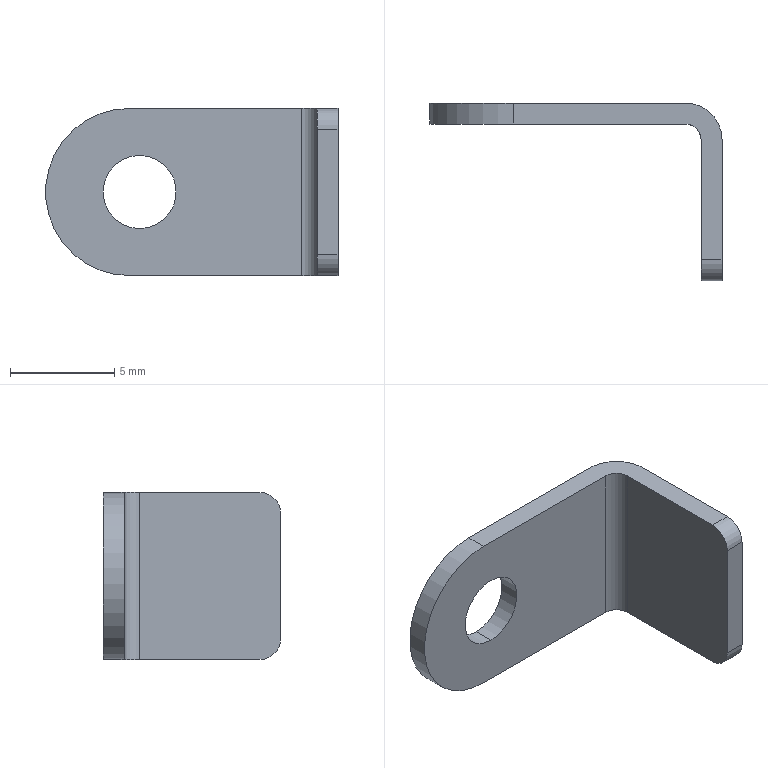Part | SolidWorks | features BaseBody 1 | 1 solid | 14 faces | box 14 x 8.5 x 8 mm | volume 150.836 mm3 | cylinder 7 | plane 7 | commonest cylinder face diameters 2 x2 3.5 x2 1.473 x1 3.473 x1 8 x1
STEP:
#1=CARTESIAN_POINT('',(-2.5,-1.,1.75));
#2=VERTEX_POINT('',#1);
#3=CARTESIAN_POINT('',(-2.5,-1.,-1.75));
#4=VERTEX_POINT('',#3);
#5=CARTESIAN_POINT('',(-2.5,-1.,0.));
#6=DIRECTION('',(0.,-1.,0.));
#7=DIRECTION('',(0.,0.,1.));
#8=AXIS2_PLACEMENT_3D('',#5,#6,#7);
#9=CIRCLE('',#8,1.75);
#10=EDGE_CURVE('',#2,#4,#9,.T.);
#11=ORIENTED_EDGE('',*,*,#10,.T.);
#12=CARTESIAN_POINT('',(-2.5,0.,-1.75));
#13=VERTEX_POINT('',#12);
#14=CARTESIAN_POINT('',(-2.5,-1.,-1.75));
#15=DIRECTION('',(0.,1.,0.));
#16=VECTOR('',#15,1000.);
#17=LINE('',#14,#16);
#18=EDGE_CURVE('',#4,#13,#17,.T.);
#19=ORIENTED_EDGE('',*,*,#18,.T.);
#20=CARTESIAN_POINT('',(-2.5,0.,1.75));
#21=VERTEX_POINT('',#20);
#22=CARTESIAN_POINT('',(-2.5,0.,0.));
#23=DIRECTION('',(0.,-1.,0.));
#24=DIRECTION('',(0.,0.,1.));
#25=AXIS2_PLACEMENT_3D('',#22,#23,#24);
#26=CIRCLE('',#25,1.75);
#27=EDGE_CURVE('',#21,#13,#26,.T.);
#28=ORIENTED_EDGE('',*,*,#27,.F.);
#29=CARTESIAN_POINT('',(-2.5,-1.,1.75));
#30=DIRECTION('',(0.,1.,0.));
#31=VECTOR('',#30,1000.);
#32=LINE('',#29,#31);
#33=EDGE_CURVE('',#2,#21,#32,.T.);
#34=ORIENTED_EDGE('',*,*,#33,.F.);
#35=EDGE_LOOP('',(#11,#19,#28,#34));
#36=FACE_OUTER_BOUND('',#35,.T.);
#37=CARTESIAN_POINT('',(-2.5,-1.,0.));
#38=DIRECTION('',(0.,1.,0.));
#39=DIRECTION('',(0.,0.,1.));
#40=AXIS2_PLACEMENT_3D('',#37,#38,#39);
#41=CYLINDRICAL_SURFACE('',#40,1.75);
#42=ADVANCED_FACE('',(#36),#41,.F.);
#43=CARTESIAN_POINT('',(-3.,-1.,4.));
#44=VERTEX_POINT('',#43);
#45=CARTESIAN_POINT('',(5.263,-1.,4.));
#46=VERTEX_POINT('',#45);
#47=CARTESIAN_POINT('',(-7.,-1.,4.));
#48=DIRECTION('',(1.,0.,0.));
#49=VECTOR('',#48,1000.);
#50=LINE('',#47,#49);
#51=EDGE_CURVE('',#44,#46,#50,.T.);
#52=ORIENTED_EDGE('',*,*,#51,.F.);
#53=CARTESIAN_POINT('',(-3.,-1.,-4.));
#54=VERTEX_POINT('',#53);
#55=CARTESIAN_POINT('',(-3.,-1.,0.));
#56=DIRECTION('',(0.,1.,0.));
#57=DIRECTION('',(0.,0.,1.));
#58=AXIS2_PLACEMENT_3D('',#55,#56,#57);
#59=CIRCLE('',#58,4.);
#60=EDGE_CURVE('',#54,#44,#59,.T.);
#61=ORIENTED_EDGE('',*,*,#60,.F.);
#62=CARTESIAN_POINT('',(5.263,-1.,-4.));
#63=VERTEX_POINT('',#62);
#64=CARTESIAN_POINT('',(-7.,-1.,-4.));
#65=DIRECTION('',(-1.,0.,0.));
#66=VECTOR('',#65,1000.);
#67=LINE('',#64,#66);
#68=EDGE_CURVE('',#63,#54,#67,.T.);
#69=ORIENTED_EDGE('',*,*,#68,.F.);
#70=CARTESIAN_POINT('',(5.263,-1.,4.));
#71=DIRECTION('',(0.,0.,-1.));
#72=VECTOR('',#71,1000.);
#73=LINE('',#70,#72);
#74=EDGE_CURVE('',#46,#63,#73,.T.);
#75=ORIENTED_EDGE('',*,*,#74,.F.);
#76=EDGE_LOOP('',(#52,#61,#69,#75));
#77=FACE_OUTER_BOUND('',#76,.T.);
#78=ORIENTED_EDGE('',*,*,#10,.F.);
#79=CARTESIAN_POINT('',(-2.5,-1.,0.));
#80=DIRECTION('',(0.,-1.,0.));
#81=DIRECTION('',(0.,0.,1.));
#82=AXIS2_PLACEMENT_3D('',#79,#80,#81);
#83=CIRCLE('',#82,1.75);
#84=EDGE_CURVE('',#4,#2,#83,.T.);
#85=ORIENTED_EDGE('',*,*,#84,.F.);
#86=EDGE_LOOP('',(#78,#85));
#87=FACE_BOUND('',#86,.T.);
#88=CARTESIAN_POINT('',(-7.,-1.,4.));
#89=DIRECTION('',(0.,1.,0.));
#90=DIRECTION('',(0.,0.,1.));
#91=AXIS2_PLACEMENT_3D('',#88,#89,#90);
#92=PLANE('',#91);
#93=ADVANCED_FACE('',(#77,#87),#92,.F.);
#94=CARTESIAN_POINT('',(6.,-1.737,-4.));
#95=VERTEX_POINT('',#94);
#96=CARTESIAN_POINT('',(5.263,-1.737,-4.));
#97=DIRECTION('',(0.,0.,1.));
#98=DIRECTION('',(1.,0.,0.));
#99=AXIS2_PLACEMENT_3D('',#96,#97,#98);
#100=CIRCLE('',#99,0.7366);
#101=EDGE_CURVE('',#95,#63,#100,.T.);
#102=ORIENTED_EDGE('',*,*,#101,.F.);
#103=CARTESIAN_POINT('',(6.,-1.737,4.));
#104=VERTEX_POINT('',#103);
#105=CARTESIAN_POINT('',(6.,-1.737,4.));
#106=DIRECTION('',(0.,0.,-1.));
#107=VECTOR('',#106,1000.);
#108=LINE('',#105,#107);
#109=EDGE_CURVE('',#104,#95,#108,.T.);
#110=ORIENTED_EDGE('',*,*,#109,.F.);
#111=CARTESIAN_POINT('',(5.263,-1.737,4.));
#112=DIRECTION('',(0.,0.,1.));
#113=DIRECTION('',(1.,0.,0.));
#114=AXIS2_PLACEMENT_3D('',#111,#112,#113);
#115=CIRCLE('',#114,0.7366);
#116=EDGE_CURVE('',#104,#46,#115,.T.);
#117=ORIENTED_EDGE('',*,*,#116,.T.);
#118=ORIENTED_EDGE('',*,*,#74,.T.);
#119=EDGE_LOOP('',(#102,#110,#117,#118));
#120=FACE_OUTER_BOUND('',#119,.T.);
#121=CARTESIAN_POINT('',(5.263,-1.737,4.));
#122=DIRECTION('',(0.,0.,1.));
#123=DIRECTION('',(1.,0.,0.));
#124=AXIS2_PLACEMENT_3D('',#121,#122,#123);
#125=CYLINDRICAL_SURFACE('',#124,0.7366);
#126=ADVANCED_FACE('',(#120),#125,.F.);
#127=CARTESIAN_POINT('',(-3.,0.,4.));
#128=VERTEX_POINT('',#127);
#129=CARTESIAN_POINT('',(5.263,0.,4.));
#130=VERTEX_POINT('',#129);
#131=CARTESIAN_POINT('',(0.,0.,4.));
#132=DIRECTION('',(1.,0.,0.));
#133=VECTOR('',#132,1000.);
#134=LINE('',#131,#133);
#135=EDGE_CURVE('',#128,#130,#134,.T.);
#136=ORIENTED_EDGE('',*,*,#135,.F.);
#137=CARTESIAN_POINT('',(-3.,0.,4.));
#138=DIRECTION('',(0.,1.,0.));
#139=VECTOR('',#138,1000.);
#140=LINE('',#137,#139);
#141=EDGE_CURVE('',#44,#128,#140,.T.);
#142=ORIENTED_EDGE('',*,*,#141,.F.);
#143=ORIENTED_EDGE('',*,*,#51,.T.);
#144=ORIENTED_EDGE('',*,*,#116,.F.);
#145=CARTESIAN_POINT('',(6.,-7.5,4.));
#146=VERTEX_POINT('',#145);
#147=CARTESIAN_POINT('',(6.,0.,4.));
#148=DIRECTION('',(0.,1.,0.));
#149=VECTOR('',#148,1000.);
#150=LINE('',#147,#149);
#151=EDGE_CURVE('',#146,#104,#150,.T.);
#152=ORIENTED_EDGE('',*,*,#151,.F.);
#153=CARTESIAN_POINT('',(7.,-7.5,4.));
#154=VERTEX_POINT('',#153);
#155=CARTESIAN_POINT('',(7.,-7.5,4.));
#156=DIRECTION('',(-1.,0.,0.));
#157=VECTOR('',#156,1000.);
#158=LINE('',#155,#157);
#159=EDGE_CURVE('',#154,#146,#158,.T.);
#160=ORIENTED_EDGE('',*,*,#159,.F.);
#161=CARTESIAN_POINT('',(7.,-1.737,4.));
#162=VERTEX_POINT('',#161);
#163=CARTESIAN_POINT('',(7.,-8.5,4.));
#164=DIRECTION('',(0.,-1.,0.));
#165=VECTOR('',#164,1000.);
#166=LINE('',#163,#165);
#167=EDGE_CURVE('',#162,#154,#166,.T.);
#168=ORIENTED_EDGE('',*,*,#167,.F.);
#169=CARTESIAN_POINT('',(5.263,-1.737,4.));
#170=DIRECTION('',(0.,0.,-1.));
#171=DIRECTION('',(1.,0.,0.));
#172=AXIS2_PLACEMENT_3D('',#169,#170,#171);
#173=CIRCLE('',#172,1.737);
#174=EDGE_CURVE('',#130,#162,#173,.T.);
#175=ORIENTED_EDGE('',*,*,#174,.F.);
#176=EDGE_LOOP('',(#136,#142,#143,#144,#152,#160,#168,#175));
#177=FACE_OUTER_BOUND('',#176,.T.);
#178=CARTESIAN_POINT('',(0.,0.,4.));
#179=DIRECTION('',(0.,0.,-1.));
#180=DIRECTION('',(-1.,0.,0.));
#181=AXIS2_PLACEMENT_3D('',#178,#179,#180);
#182=PLANE('',#181);
#183=ADVANCED_FACE('',(#177),#182,.F.);
#184=ORIENTED_EDGE('',*,*,#141,.T.);
#185=CARTESIAN_POINT('',(-3.,0.,-4.));
#186=VERTEX_POINT('',#185);
#187=CARTESIAN_POINT('',(-3.,0.,0.));
#188=DIRECTION('',(0.,-1.,0.));
#189=DIRECTION('',(0.,0.,-1.));
#190=AXIS2_PLACEMENT_3D('',#187,#188,#189);
#191=CIRCLE('',#190,4.);
#192=EDGE_CURVE('',#128,#186,#191,.T.);
#193=ORIENTED_EDGE('',*,*,#192,.T.);
#194=CARTESIAN_POINT('',(-3.,0.,-4.));
#195=DIRECTION('',(0.,-1.,0.));
#196=VECTOR('',#195,1000.);
#197=LINE('',#194,#196);
#198=EDGE_CURVE('',#186,#54,#197,.T.);
#199=ORIENTED_EDGE('',*,*,#198,.T.);
#200=ORIENTED_EDGE('',*,*,#60,.T.);
#201=EDGE_LOOP('',(#184,#193,#199,#200));
#202=FACE_OUTER_BOUND('',#201,.T.);
#203=CARTESIAN_POINT('',(-3.,-1.,0.));
#204=DIRECTION('',(0.,-1.,0.));
#205=DIRECTION('',(0.,0.,-1.));
#206=AXIS2_PLACEMENT_3D('',#203,#204,#205);
#207=CYLINDRICAL_SURFACE('',#206,4.);
#208=ADVANCED_FACE('',(#202),#207,.T.);
#209=ORIENTED_EDGE('',*,*,#198,.F.);
#210=CARTESIAN_POINT('',(5.263,0.,-4.));
#211=VERTEX_POINT('',#210);
#212=CARTESIAN_POINT('',(0.,0.,-4.));
#213=DIRECTION('',(1.,0.,0.));
#214=VECTOR('',#213,1000.);
#215=LINE('',#212,#214);
#216=EDGE_CURVE('',#186,#211,#215,.T.);
#217=ORIENTED_EDGE('',*,*,#216,.T.);
#218=CARTESIAN_POINT('',(7.,-1.737,-4.));
#219=VERTEX_POINT('',#218);
#220=CARTESIAN_POINT('',(5.263,-1.737,-4.));
#221=DIRECTION('',(0.,0.,1.));
#222=DIRECTION('',(1.,0.,0.));
#223=AXIS2_PLACEMENT_3D('',#220,#221,#222);
#224=CIRCLE('',#223,1.737);
#225=EDGE_CURVE('',#219,#211,#224,.T.);
#226=ORIENTED_EDGE('',*,*,#225,.F.);
#227=CARTESIAN_POINT('',(7.,-7.5,-4.));
#228=VERTEX_POINT('',#227);
#229=CARTESIAN_POINT('',(7.,-1.,-4.));
#230=DIRECTION('',(0.,1.,0.));
#231=VECTOR('',#230,1000.);
#232=LINE('',#229,#231);
#233=EDGE_CURVE('',#228,#219,#232,.T.);
#234=ORIENTED_EDGE('',*,*,#233,.F.);
#235=CARTESIAN_POINT('',(6.,-7.5,-4.));
#236=VERTEX_POINT('',#235);
#237=CARTESIAN_POINT('',(7.,-7.5,-4.));
#238=DIRECTION('',(1.,0.,0.));
#239=VECTOR('',#238,1000.);
#240=LINE('',#237,#239);
#241=EDGE_CURVE('',#236,#228,#240,.T.);
#242=ORIENTED_EDGE('',*,*,#241,.F.);
#243=CARTESIAN_POINT('',(6.,0.,-4.));
#244=DIRECTION('',(0.,-1.,0.));
#245=VECTOR('',#244,1000.);
#246=LINE('',#243,#245);
#247=EDGE_CURVE('',#95,#236,#246,.T.);
#248=ORIENTED_EDGE('',*,*,#247,.F.);
#249=ORIENTED_EDGE('',*,*,#101,.T.);
#250=ORIENTED_EDGE('',*,*,#68,.T.);
#251=EDGE_LOOP('',(#209,#217,#226,#234,#242,#248,#249,#250));
#252=FACE_OUTER_BOUND('',#251,.T.);
#253=CARTESIAN_POINT('',(0.,0.,-4.));
#254=DIRECTION('',(0.,0.,-1.));
#255=DIRECTION('',(-1.,0.,0.));
#256=AXIS2_PLACEMENT_3D('',#253,#254,#255);
#257=PLANE('',#256);
#258=ADVANCED_FACE('',(#252),#257,.T.);
#259=ORIENTED_EDGE('',*,*,#18,.F.);
#260=ORIENTED_EDGE('',*,*,#84,.T.);
#261=ORIENTED_EDGE('',*,*,#33,.T.);
#262=CARTESIAN_POINT('',(-2.5,0.,0.));
#263=DIRECTION('',(0.,-1.,0.));
#264=DIRECTION('',(0.,0.,1.));
#265=AXIS2_PLACEMENT_3D('',#262,#263,#264);
#266=CIRCLE('',#265,1.75);
#267=EDGE_CURVE('',#13,#21,#266,.T.);
#268=ORIENTED_EDGE('',*,*,#267,.F.);
#269=EDGE_LOOP('',(#259,#260,#261,#268));
#270=FACE_OUTER_BOUND('',#269,.T.);
#271=CARTESIAN_POINT('',(-2.5,-1.,0.));
#272=DIRECTION('',(0.,1.,0.));
#273=DIRECTION('',(0.,0.,1.));
#274=AXIS2_PLACEMENT_3D('',#271,#272,#273);
#275=CYLINDRICAL_SURFACE('',#274,1.75);
#276=ADVANCED_FACE('',(#270),#275,.F.);
#277=ORIENTED_EDGE('',*,*,#247,.T.);
#278=CARTESIAN_POINT('',(6.,-8.5,-3.));
#279=VERTEX_POINT('',#278);
#280=CARTESIAN_POINT('',(6.,-7.5,-3.));
#281=DIRECTION('',(-1.,0.,0.));
#282=DIRECTION('',(0.,-1.,0.));
#283=AXIS2_PLACEMENT_3D('',#280,#281,#282);
#284=CIRCLE('',#283,1.);
#285=EDGE_CURVE('',#236,#279,#284,.T.);
#286=ORIENTED_EDGE('',*,*,#285,.T.);
#287=CARTESIAN_POINT('',(6.,-8.5,3.));
#288=VERTEX_POINT('',#287);
#289=CARTESIAN_POINT('',(6.,-8.5,0.));
#290=DIRECTION('',(0.,0.,1.));
#291=VECTOR('',#290,1000.);
#292=LINE('',#289,#291);
#293=EDGE_CURVE('',#279,#288,#292,.T.);
#294=ORIENTED_EDGE('',*,*,#293,.T.);
#295=CARTESIAN_POINT('',(6.,-7.5,3.));
#296=DIRECTION('',(-1.,0.,0.));
#297=DIRECTION('',(0.,-1.,0.));
#298=AXIS2_PLACEMENT_3D('',#295,#296,#297);
#299=CIRCLE('',#298,1.);
#300=EDGE_CURVE('',#288,#146,#299,.T.);
#301=ORIENTED_EDGE('',*,*,#300,.T.);
#302=ORIENTED_EDGE('',*,*,#151,.T.);
#303=ORIENTED_EDGE('',*,*,#109,.T.);
#304=EDGE_LOOP('',(#277,#286,#294,#301,#302,#303));
#305=FACE_OUTER_BOUND('',#304,.T.);
#306=CARTESIAN_POINT('',(6.,0.,0.));
#307=DIRECTION('',(-1.,0.,0.));
#308=DIRECTION('',(0.,-1.,0.));
#309=AXIS2_PLACEMENT_3D('',#306,#307,#308);
#310=PLANE('',#309);
#311=ADVANCED_FACE('',(#305),#310,.T.);
#312=ORIENTED_EDGE('',*,*,#216,.F.);
#313=ORIENTED_EDGE('',*,*,#192,.F.);
#314=ORIENTED_EDGE('',*,*,#135,.T.);
#315=CARTESIAN_POINT('',(5.263,0.,4.));
#316=DIRECTION('',(0.,0.,-1.));
#317=VECTOR('',#316,1000.);
#318=LINE('',#315,#317);
#319=EDGE_CURVE('',#130,#211,#318,.T.);
#320=ORIENTED_EDGE('',*,*,#319,.T.);
#321=EDGE_LOOP('',(#312,#313,#314,#320));
#322=FACE_OUTER_BOUND('',#321,.T.);
#323=ORIENTED_EDGE('',*,*,#27,.T.);
#324=ORIENTED_EDGE('',*,*,#267,.T.);
#325=EDGE_LOOP('',(#323,#324));
#326=FACE_BOUND('',#325,.T.);
#327=CARTESIAN_POINT('',(-7.,0.,4.));
#328=DIRECTION('',(0.,1.,0.));
#329=DIRECTION('',(0.,0.,1.));
#330=AXIS2_PLACEMENT_3D('',#327,#328,#329);
#331=PLANE('',#330);
#332=ADVANCED_FACE('',(#322,#326),#331,.T.);
#333=ORIENTED_EDGE('',*,*,#285,.F.);
#334=ORIENTED_EDGE('',*,*,#241,.T.);
#335=CARTESIAN_POINT('',(7.,-8.5,-3.));
#336=VERTEX_POINT('',#335);
#337=CARTESIAN_POINT('',(7.,-7.5,-3.));
#338=DIRECTION('',(-1.,0.,0.));
#339=DIRECTION('',(0.,-1.,0.));
#340=AXIS2_PLACEMENT_3D('',#337,#338,#339);
#341=CIRCLE('',#340,1.);
#342=EDGE_CURVE('',#228,#336,#341,.T.);
#343=ORIENTED_EDGE('',*,*,#342,.T.);
#344=CARTESIAN_POINT('',(7.,-8.5,-3.));
#345=DIRECTION('',(-1.,0.,0.));
#346=VECTOR('',#345,1000.);
#347=LINE('',#344,#346);
#348=EDGE_CURVE('',#336,#279,#347,.T.);
#349=ORIENTED_EDGE('',*,*,#348,.T.);
#350=EDGE_LOOP('',(#333,#334,#343,#349));
#351=FACE_OUTER_BOUND('',#350,.T.);
#352=CARTESIAN_POINT('',(7.,-7.5,-3.));
#353=DIRECTION('',(-1.,0.,0.));
#354=DIRECTION('',(0.,-1.,0.));
#355=AXIS2_PLACEMENT_3D('',#352,#353,#354);
#356=CYLINDRICAL_SURFACE('',#355,1.);
#357=ADVANCED_FACE('',(#351),#356,.T.);
#358=ORIENTED_EDGE('',*,*,#300,.F.);
#359=CARTESIAN_POINT('',(7.,-8.5,3.));
#360=VERTEX_POINT('',#359);
#361=CARTESIAN_POINT('',(7.,-8.5,3.));
#362=DIRECTION('',(1.,0.,0.));
#363=VECTOR('',#362,1000.);
#364=LINE('',#361,#363);
#365=EDGE_CURVE('',#288,#360,#364,.T.);
#366=ORIENTED_EDGE('',*,*,#365,.T.);
#367=CARTESIAN_POINT('',(7.,-7.5,3.));
#368=DIRECTION('',(-1.,0.,0.));
#369=DIRECTION('',(0.,-1.,0.));
#370=AXIS2_PLACEMENT_3D('',#367,#368,#369);
#371=CIRCLE('',#370,1.);
#372=EDGE_CURVE('',#360,#154,#371,.T.);
#373=ORIENTED_EDGE('',*,*,#372,.T.);
#374=ORIENTED_EDGE('',*,*,#159,.T.);
#375=EDGE_LOOP('',(#358,#366,#373,#374));
#376=FACE_OUTER_BOUND('',#375,.T.);
#377=CARTESIAN_POINT('',(7.,-7.5,3.));
#378=DIRECTION('',(-1.,0.,0.));
#379=DIRECTION('',(0.,-1.,0.));
#380=AXIS2_PLACEMENT_3D('',#377,#378,#379);
#381=CYLINDRICAL_SURFACE('',#380,1.);
#382=ADVANCED_FACE('',(#376),#381,.T.);
#383=ORIENTED_EDGE('',*,*,#365,.F.);
#384=ORIENTED_EDGE('',*,*,#293,.F.);
#385=ORIENTED_EDGE('',*,*,#348,.F.);
#386=CARTESIAN_POINT('',(7.,-8.5,-4.));
#387=DIRECTION('',(0.,0.,-1.));
#388=VECTOR('',#387,1000.);
#389=LINE('',#386,#388);
#390=EDGE_CURVE('',#360,#336,#389,.T.);
#391=ORIENTED_EDGE('',*,*,#390,.F.);
#392=EDGE_LOOP('',(#383,#384,#385,#391));
#393=FACE_OUTER_BOUND('',#392,.T.);
#394=CARTESIAN_POINT('',(7.,-8.5,-4.));
#395=DIRECTION('',(0.,1.,0.));
#396=DIRECTION('',(-1.,0.,0.));
#397=AXIS2_PLACEMENT_3D('',#394,#395,#396);
#398=PLANE('',#397);
#399=ADVANCED_FACE('',(#393),#398,.F.);
#400=CARTESIAN_POINT('',(7.,-1.737,4.));
#401=DIRECTION('',(0.,0.,-1.));
#402=VECTOR('',#401,1000.);
#403=LINE('',#400,#402);
#404=EDGE_CURVE('',#162,#219,#403,.T.);
#405=ORIENTED_EDGE('',*,*,#404,.T.);
#406=ORIENTED_EDGE('',*,*,#225,.T.);
#407=ORIENTED_EDGE('',*,*,#319,.F.);
#408=ORIENTED_EDGE('',*,*,#174,.T.);
#409=EDGE_LOOP('',(#405,#406,#407,#408));
#410=FACE_OUTER_BOUND('',#409,.T.);
#411=CARTESIAN_POINT('',(5.263,-1.737,4.));
#412=DIRECTION('',(0.,0.,1.));
#413=DIRECTION('',(1.,0.,0.));
#414=AXIS2_PLACEMENT_3D('',#411,#412,#413);
#415=CYLINDRICAL_SURFACE('',#414,1.737);
#416=ADVANCED_FACE('',(#410),#415,.T.);
#417=ORIENTED_EDGE('',*,*,#372,.F.);
#418=ORIENTED_EDGE('',*,*,#390,.T.);
#419=ORIENTED_EDGE('',*,*,#342,.F.);
#420=ORIENTED_EDGE('',*,*,#233,.T.);
#421=ORIENTED_EDGE('',*,*,#404,.F.);
#422=ORIENTED_EDGE('',*,*,#167,.T.);
#423=EDGE_LOOP('',(#417,#418,#419,#420,#421,#422));
#424=FACE_OUTER_BOUND('',#423,.T.);
#425=CARTESIAN_POINT('',(7.,0.,0.));
#426=DIRECTION('',(-1.,0.,0.));
#427=DIRECTION('',(0.,-1.,0.));
#428=AXIS2_PLACEMENT_3D('',#425,#426,#427);
#429=PLANE('',#428);
#430=ADVANCED_FACE('',(#424),#429,.F.);
#431=CLOSED_SHELL('',(#42,#93,#126,#183,#208,#258,#276,#311,#332,#357,#382,#399,#416,#430));
#432=MANIFOLD_SOLID_BREP('',#431);
#433=CARTESIAN_POINT('',(0.,0.,0.));
#434=DIRECTION('',(0.,0.,1.));
#435=DIRECTION('',(1.,0.,0.));
#436=AXIS2_PLACEMENT_3D('',#433,#434,#435);
#437=(LENGTH_UNIT()NAMED_UNIT(*)SI_UNIT(.MILLI.,.METRE.));
#438=UNCERTAINTY_MEASURE_WITH_UNIT(LENGTH_MEASURE(0.00001),#437,'','');
#439=(NAMED_UNIT(*)PLANE_ANGLE_UNIT()SI_UNIT($,.RADIAN.));
#440=(NAMED_UNIT(*)SI_UNIT($,.STERADIAN.)SOLID_ANGLE_UNIT());
#441=(GEOMETRIC_REPRESENTATION_CONTEXT(3)GLOBAL_UNCERTAINTY_ASSIGNED_CONTEXT((#438))GLOBAL_UNIT_ASSIGNED_CONTEXT((#437,#439,#440))REPRESENTATION_CONTEXT('',''));
#442=ADVANCED_BREP_SHAPE_REPRESENTATION('',(#432,#436),#441);